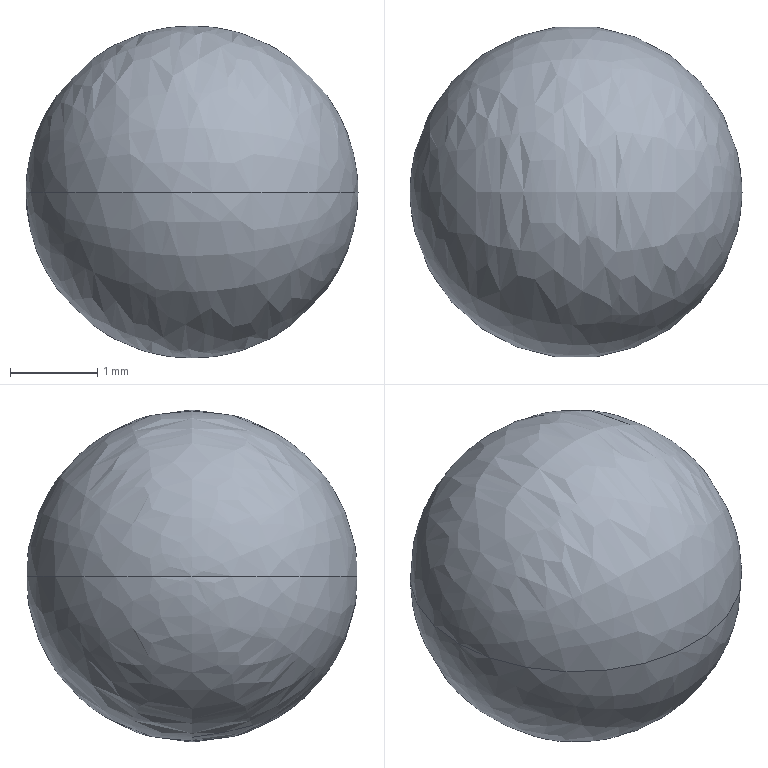Part | SolidWorks | features BaseBody 1 | 1 solid | 2 faces | volume 28.73 mm3 | spline 2
STEP:
#1=CARTESIAN_POINT('',(1.9,0.,0.));
#2=VERTEX_POINT('',#1);
#3=CARTESIAN_POINT('',(-1.9,0.,0.));
#4=VERTEX_POINT('',#3);
#5=CARTESIAN_POINT('',(0.,0.,0.));
#6=DIRECTION('',(0.,0.,1.));
#7=DIRECTION('',(1.,0.,0.));
#8=AXIS2_PLACEMENT_3D('',#5,#6,#7);
#9=CIRCLE('',#8,1.9);
#10=EDGE_CURVE('',#2,#4,#9,.T.);
#11=ORIENTED_EDGE('',*,*,#10,.F.);
#12=CARTESIAN_POINT('',(0.,0.,0.));
#13=DIRECTION('',(0.,0.,-1.));
#14=DIRECTION('',(1.,0.,0.));
#15=AXIS2_PLACEMENT_3D('',#12,#13,#14);
#16=CIRCLE('',#15,1.9);
#17=EDGE_CURVE('',#2,#4,#16,.T.);
#18=ORIENTED_EDGE('',*,*,#17,.T.);
#19=EDGE_LOOP('',(#11,#18));
#20=FACE_OUTER_BOUND('',#19,.T.);
#21=CARTESIAN_POINT('',(1.9,0.,0.));
#22=CARTESIAN_POINT('',(1.9,0.,0.));
#23=CARTESIAN_POINT('',(1.9,0.,0.));
#24=CARTESIAN_POINT('',(1.9,0.,0.));
#25=CARTESIAN_POINT('',(1.9,-3.8,0.));
#26=CARTESIAN_POINT('',(1.9,-3.8,-7.6));
#27=CARTESIAN_POINT('',(1.9,3.8,-7.6));
#28=CARTESIAN_POINT('',(1.9,3.8,0.));
#29=CARTESIAN_POINT('',(-1.9,-3.8,0.));
#30=CARTESIAN_POINT('',(-1.9,-3.8,-7.6));
#31=CARTESIAN_POINT('',(-1.9,3.8,-7.6));
#32=CARTESIAN_POINT('',(-1.9,3.8,0.));
#33=CARTESIAN_POINT('',(-1.9,0.,0.));
#34=CARTESIAN_POINT('',(-1.9,0.,0.));
#35=CARTESIAN_POINT('',(-1.9,0.,0.));
#36=CARTESIAN_POINT('',(-1.9,0.,0.));
#37=(BOUNDED_SURFACE()B_SPLINE_SURFACE(3,3,((#21,#22,#23,#24),(#25,#26,#27,#28),(#29,#30,#31,#32),(#33,#34,#35,#36)),.UNSPECIFIED.,.F.,.F.,.T.)B_SPLINE_SURFACE_WITH_KNOTS((4,4),(4,4),(0.,1.),(0.,1.),.UNSPECIFIED.)GEOMETRIC_REPRESENTATION_ITEM()RATIONAL_B_SPLINE_SURFACE(((1.,0.3333,0.3333,1.),(0.3333,0.1111,0.1111,0.3333),(0.3333,0.1111,0.1111,0.3333),(1.,0.3333,0.3333,1.)))REPRESENTATION_ITEM('')SURFACE());
#38=ADVANCED_FACE('',(#20),#37,.T.);
#39=ORIENTED_EDGE('',*,*,#17,.F.);
#40=ORIENTED_EDGE('',*,*,#10,.T.);
#41=EDGE_LOOP('',(#39,#40));
#42=FACE_OUTER_BOUND('',#41,.T.);
#43=CARTESIAN_POINT('',(1.9,0.,0.));
#44=CARTESIAN_POINT('',(1.9,0.,0.));
#45=CARTESIAN_POINT('',(1.9,0.,0.));
#46=CARTESIAN_POINT('',(1.9,0.,0.));
#47=CARTESIAN_POINT('',(1.9,3.8,0.));
#48=CARTESIAN_POINT('',(1.9,3.8,7.6));
#49=CARTESIAN_POINT('',(1.9,-3.8,7.6));
#50=CARTESIAN_POINT('',(1.9,-3.8,0.));
#51=CARTESIAN_POINT('',(-1.9,3.8,0.));
#52=CARTESIAN_POINT('',(-1.9,3.8,7.6));
#53=CARTESIAN_POINT('',(-1.9,-3.8,7.6));
#54=CARTESIAN_POINT('',(-1.9,-3.8,0.));
#55=CARTESIAN_POINT('',(-1.9,0.,0.));
#56=CARTESIAN_POINT('',(-1.9,0.,0.));
#57=CARTESIAN_POINT('',(-1.9,0.,0.));
#58=CARTESIAN_POINT('',(-1.9,0.,0.));
#59=(BOUNDED_SURFACE()B_SPLINE_SURFACE(3,3,((#43,#44,#45,#46),(#47,#48,#49,#50),(#51,#52,#53,#54),(#55,#56,#57,#58)),.UNSPECIFIED.,.F.,.F.,.F.)B_SPLINE_SURFACE_WITH_KNOTS((4,4),(4,4),(0.,1.),(0.,1.),.UNSPECIFIED.)GEOMETRIC_REPRESENTATION_ITEM()RATIONAL_B_SPLINE_SURFACE(((1.,0.3333,0.3333,1.),(0.3333,0.1111,0.1111,0.3333),(0.3333,0.1111,0.1111,0.3333),(1.,0.3333,0.3333,1.)))REPRESENTATION_ITEM('')SURFACE());
#60=ADVANCED_FACE('',(#42),#59,.T.);
#61=CLOSED_SHELL('',(#38,#60));
#62=MANIFOLD_SOLID_BREP('',#61);
#63=CARTESIAN_POINT('',(0.,0.,0.));
#64=DIRECTION('',(0.,0.,1.));
#65=DIRECTION('',(1.,0.,0.));
#66=AXIS2_PLACEMENT_3D('',#63,#64,#65);
#67=(LENGTH_UNIT()NAMED_UNIT(*)SI_UNIT(.MILLI.,.METRE.));
#68=UNCERTAINTY_MEASURE_WITH_UNIT(LENGTH_MEASURE(0.00001),#67,'','');
#69=(NAMED_UNIT(*)PLANE_ANGLE_UNIT()SI_UNIT($,.RADIAN.));
#70=(NAMED_UNIT(*)SI_UNIT($,.STERADIAN.)SOLID_ANGLE_UNIT());
#71=(GEOMETRIC_REPRESENTATION_CONTEXT(3)GLOBAL_UNCERTAINTY_ASSIGNED_CONTEXT((#68))GLOBAL_UNIT_ASSIGNED_CONTEXT((#67,#69,#70))REPRESENTATION_CONTEXT('',''));
#72=ADVANCED_BREP_SHAPE_REPRESENTATION('',(#62,#66),#71);